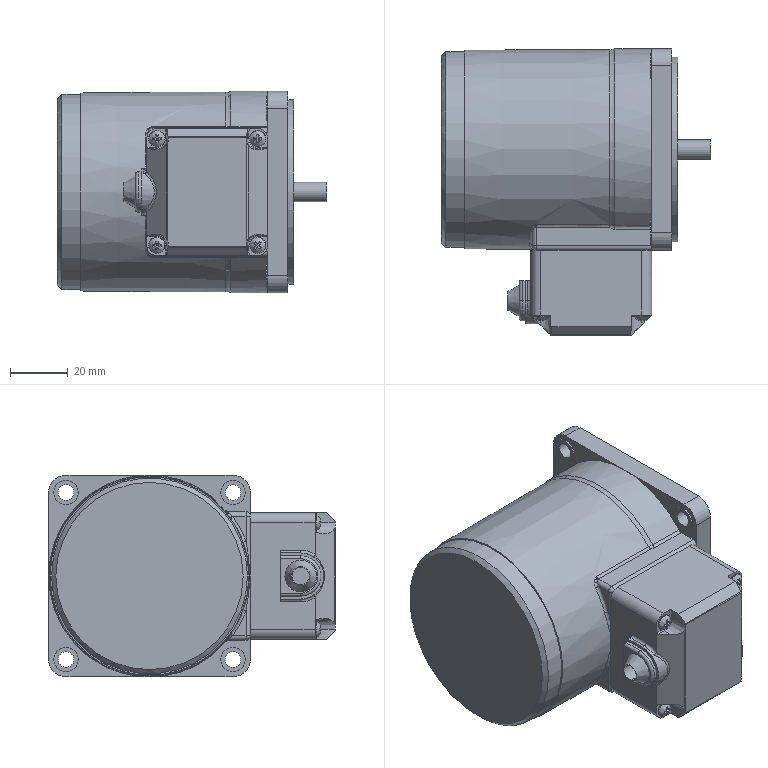Part | STEP file | S7I15G_T | 1 solid | 304 faces | box 93.4 x 99.5 x 70 mm | volume 343448 mm3 | plane 143 | cylinder 94 | spline 36 | torus 18 | cone 11 | sphere 2 | commonest cylinder face diameters 3 x15 2 x12 4 x12 1 x5 3.5 x4 3.8 x4